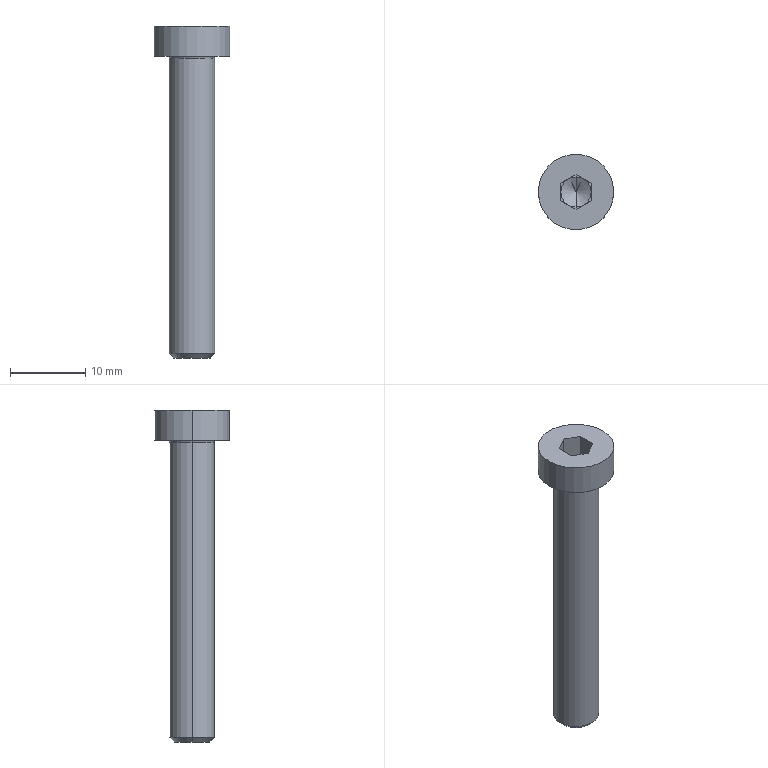Part | STEP file | TAF02-M6-L40^Motor mount assembly | 1 solid | 25 faces | box 10 x 10 x 44 mm | volume 1396 mm3 | plane 15 | cylinder 4 | cone 4 | torus 2 | commonest cylinder face diameters 6 x2 10 x2